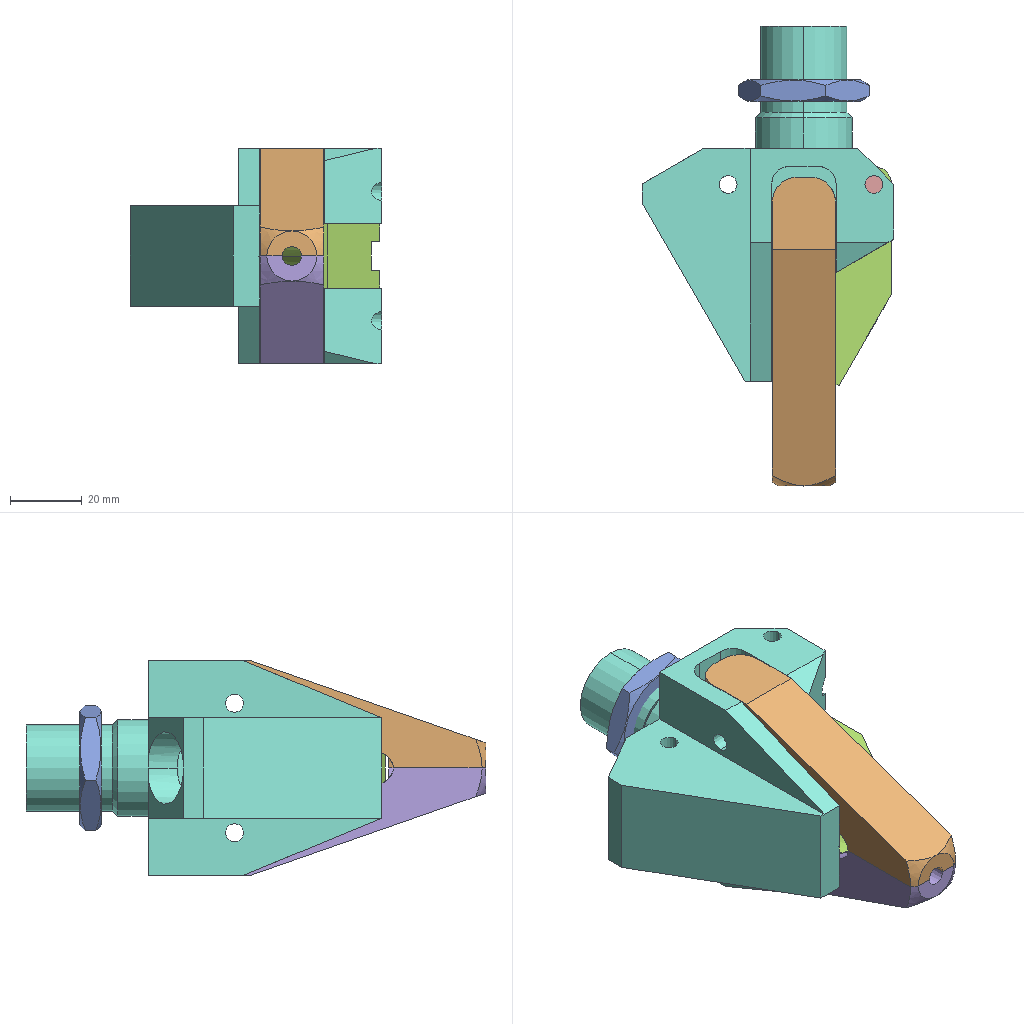Assembly | SolidWorks | 9 different items | 9 placed | box 70 x 128 x 60 mm
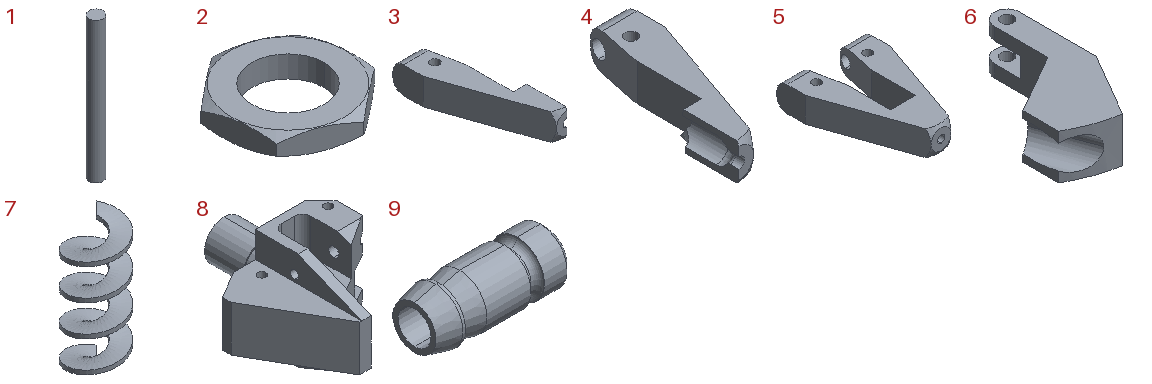Parts list (item | quantity | size | volume | features):
1 | x1 | 5 x 5 x 50 mm | 981.748 mm3 | features Extrusion 1
2 | x1 | 34.301 x 36.575 x 6 mm | 3343 mm3 | features ICE 2, Extrusion 1
3 | x1 | 30 x 86 x 17.7 mm | 18921 mm3 | features ICE 6, Extrusion 1, Fillet 1, RevCut 1
4 | x1 | 30 x 86 x 17.7 mm | 18954 mm3 | features ICE 6, Extrusion 1, Fillet 1, RevCut 1
5 | x1 | 60 x 86 x 17.7 mm | 37874 mm3 | features ICE 5, Extrusion 1, Fillet 1, RevCut 1
6 | x1 | 33.5 x 60.913 x 17.9 mm | 14389 mm3 | features ICE 3, Extrusion 1
7 | x1 | 6.243 x 6.243 x 15.5 mm | 53.36 mm3 | features Helix 1, Sweep 1
8 | x1 | 70 x 99.1 x 60 mm | 78724 mm3 | features ICE 11, Chamfer 1, Extrusion 1, Fillet 1, MirrorPattern 1
9 | x1 | 49 x 20.2 x 20.2 mm | 8256 mm3 | features ICE 1, Revolution 1
Mates (type | each side: item.copy, entity, surface, feature):
Concentric | 1.1 face cylinder Boss-Extrude1 | 8.1 face cylinder Cut-Extrude3
Width | 8.1 face plane Boss-Extrude1 | 8.1 face plane Boss-Extrude1 | 1.1 face plane Boss-Extrude1 | 1.1 face plane Boss-Extrude1
Concentric | 9.1 face cylinder Revolve1 | 8.1 face cylinder Cut-Extrude7
DistanceDim | 9.1 face plane Revolve1 | 8.1 face plane Boss-Extrude1
Concentric | 2.1 face cylinder Boss-Extrude1 | 8.1 face cylinder Boss-Extrude3
DistanceDim | 2.1 face plane Boss-Extrude1 | 8.1 face plane Boss-Extrude3
Concentric | 1.1 face cylinder Boss-Extrude1 | 6.1 face cylinder Boss-Extrude1
Width | 8.1 face plane Cut-Extrude1 | 8.1 face plane Cut-Extrude1 | 6.1 face plane Boss-Extrude1 | 6.1 face plane Boss-Extrude1
Parallel | 6.1 face plane Boss-Extrude1 | 8.1 face plane Boss-Extrude1
Coincident | 3.1 face plane Cut-Extrude7 | 4.1 face plane Cut-Extrude8
Coincident | 3.1 face plane Boss-Extrude2 | 4.1 face plane Boss-Extrude2 | 2 times
Width | 8.1 face plane Boss-Extrude1 | 8.1 face plane Boss-Extrude1 | 3.1 face plane Boss-Extrude2 | 4.1 face plane Boss-Extrude2
DistanceDim | 3.1 face plane Boss-Extrude2 | 8.1 face plane Cut-Extrude2
Width | 8.1 face plane Cut-Extrude2 | 8.1 face plane Boss-Extrude1 | 3.1 face plane Boss-Extrude2 | 3.1 face plane Boss-Extrude2